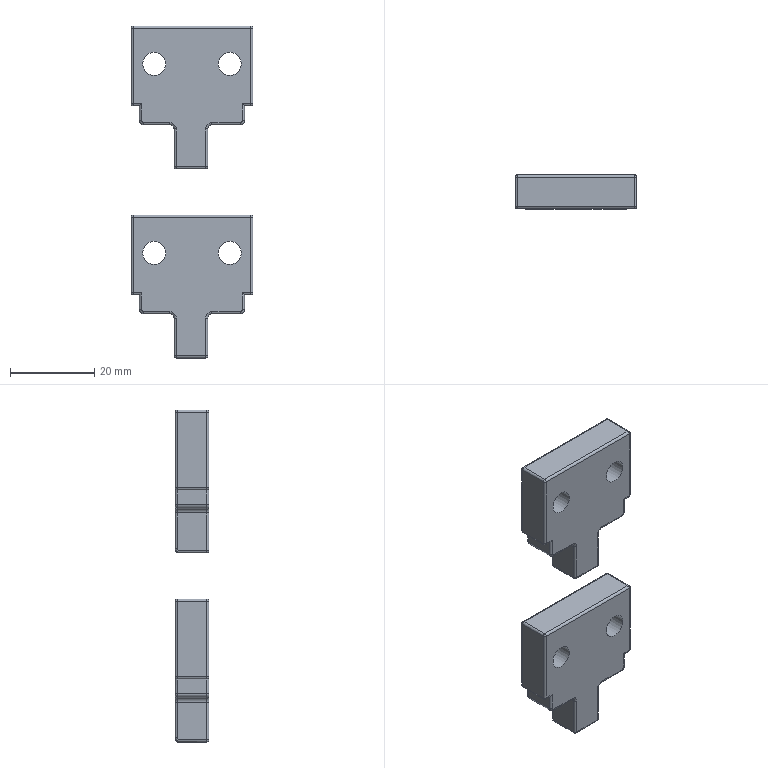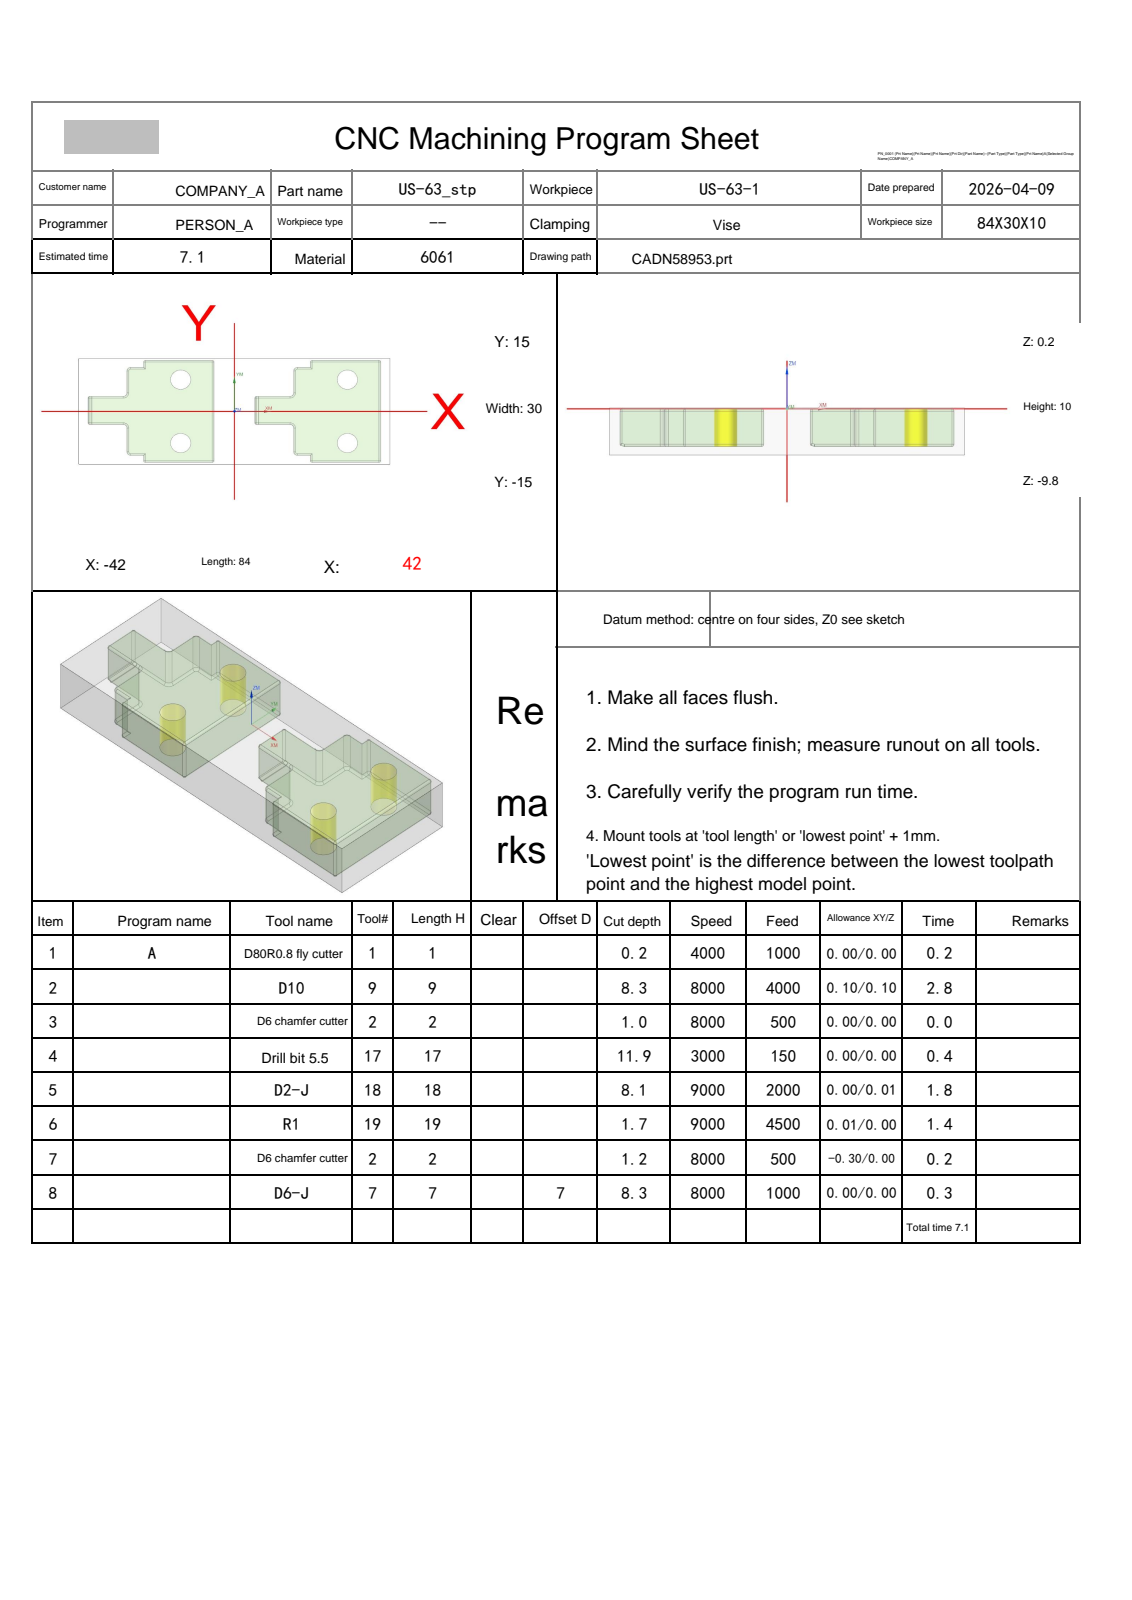NC program | NX | posted by the shop | part box 29 x 8 x 79 mm
Lines 2455 to 3429 of 24039:
N5 T18 M06
(D2-J  D=2. R=0. H=18 ce=0.00 di=0.01)
G00 G90 G54 X-24.921 Y-15.377 M03 S9000
G43 H18 Z20.
M08
Z.279
G01 X-24.92 Y-15.375 Z.232 F1600.
X-24.915 Y-15.367 Z.184
X-24.909 Y-15.355 Z.138
X-24.901 Y-15.339 Z.092
X-24.893 Y-15.319 Z.049
X-24.884 Y-15.297 Z.007
X-24.876 Y-15.272 Z-.031
X-24.869 Y-15.246 Z-.067
X-24.865 Y-15.219 Z-.1
X-24.863 Y-15.191 Z-.128
X-24.864 Y-15.163 Z-.152
X-24.869 Y-15.136 Z-.172
X-24.879 Y-15.11 Z-.187
X-24.894 Y-15.086 Z-.196
X-24.915 Y-15.063 Z-.199
G02 X-25.403 Y-14. I.915 J1.063 F2000.
G01 Y-13.403
X-28.
G02 X-28.256 Y-13.385 I0.0 J1.903
G01 X-28.273 Y-13.394 Z-.197
X-28.257 Y-13.426 Z-.193
X-28.213 Y-13.478 Z-.186
X-28.144 Y-13.548 Z-.178
X-28.052 Y-13.633 Z-.17
X-27.869 Y-13.785 Z-.159
X-27.735 Y-13.89 Z-.154
X-27.516 Y-14.051 Z-.151
X-27.144 Y-14.294 Z-.161
X-26.746 Y-14.522 Z-.187
X-26.337 Y-14.726 Z-.223
X-25.93 Y-14.897 Z-.267
X-25.676 Y-14.985 Z-.297
X-25.515 Y-15.035 Z-.317
X-25.289 Y-15.096 Z-.347
X-25.168 Y-15.123 Z-.363
X-25.073 Y-15.139 Z-.377
X-25.007 Y-15.145 Z-.388
X-24.974 Y-15.14 Z-.395
X-24.979 Y-15.124 Z-.398
G02 X-25.49 Y-14. I.979 J1.124
G01 Y-13.49
X-28.
G02 X-28.286 Y-13.47 I0.0 J1.99
G01 X-28.302 Y-13.478
X-28.287 Y-13.511
X-28.242 Y-13.565 Z-.399
X-28.172 Y-13.637 Z-.401
X-28.078 Y-13.724 Z-.403
X-27.893 Y-13.878 Z-.409
X-27.758 Y-13.984 Z-.414
X-27.535 Y-14.145 Z-.423
X-27.157 Y-14.385 Z-.444
X-26.753 Y-14.605 Z-.469
X-26.336 Y-14.798 Z-.498
X-25.923 Y-14.957 Z-.526
X-25.664 Y-15.038 Z-.544
X-25.501 Y-15.083 Z-.555
X-25.271 Y-15.137 Z-.571
X-25.149 Y-15.16 Z-.58
X-25.053 Y-15.173 Z-.587
X-24.985 Y-15.177 Z-.592
X-24.952 Y-15.171 Z-.595
X-24.957 Y-15.155 Z-.596
G02 X-25.5 Y-14. I.957 J1.155
G01 Y-13.5
X-28.
G02 X-28.284 Y-13.48 I0.0 J2.
G01 X-28.3 Y-13.486 Z-.597
X-28.29 Y-13.513 Z-.599
X-28.257 Y-13.557 Z-.602
X-28.201 Y-13.617 Z-.607
X-28.126 Y-13.689 Z-.612
X-27.924 Y-13.862 Z-.626
X-27.782 Y-13.975 Z-.635
X-27.534 Y-14.156 Z-.65
X-27.156 Y-14.394 Z-.672
X-26.752 Y-14.613 Z-.696
X-26.336 Y-14.805 Z-.719
X-25.922 Y-14.962 Z-.741
X-25.664 Y-15.042 Z-.755
X-25.501 Y-15.086 Z-.763
X-25.271 Y-15.139 Z-.776
X-25.149 Y-15.161 Z-.782
X-25.052 Y-15.174 Z-.787
X-24.985 Y-15.177 Z-.792
X-24.952 Y-15.171 Z-.794
X-24.957 Y-15.155 Z-.795
G02 X-25.5 Y-14. I.957 J1.155
G01 Y-13.5
X-28.
G02 X-28.285 Y-13.48 I0.0 J2.
G01 X-28.301 Y-13.486 Z-.796
X-28.291 Y-13.513 Z-.798
X-28.257 Y-13.557 Z-.801
X-28.201 Y-13.617 Z-.806
X-28.126 Y-13.689 Z-.811
X-27.925 Y-13.862 Z-.824
X-27.782 Y-13.975 Z-.834
X-27.534 Y-14.156 Z-.849
X-27.156 Y-14.394 Z-.871
X-26.752 Y-14.613 Z-.894
X-26.336 Y-14.805 Z-.918
X-25.922 Y-14.962 Z-.94
X-25.664 Y-15.042 Z-.954
X-25.501 Y-15.086 Z-.962
X-25.271 Y-15.139 Z-.974
X-25.149 Y-15.161 Z-.981
X-25.052 Y-15.174 Z-.986
X-24.985 Y-15.178 Z-.99
X-24.952 Y-15.171 Z-.993
X-24.957 Y-15.155 Z-.994
G02 X-25.5 Y-14. I.957 J1.155
G01 Y-13.5
X-28.
G02 X-28.285 Y-13.48 I0.0 J2.
G01 X-28.301 Y-13.486
X-28.291 Y-13.513 Z-.997
X-28.257 Y-13.557 Z-1.
X-28.201 Y-13.617 Z-1.004
X-28.126 Y-13.689 Z-1.01
X-27.925 Y-13.862 Z-1.023
X-27.782 Y-13.975 Z-1.032
X-27.534 Y-14.156 Z-1.048
X-27.156 Y-14.394 Z-1.07
X-26.752 Y-14.613 Z-1.093
X-26.336 Y-14.805 Z-1.116
X-25.922 Y-14.962 Z-1.139
X-25.664 Y-15.042 Z-1.152
X-25.501 Y-15.086 Z-1.161
X-25.271 Y-15.139 Z-1.173
X-25.149 Y-15.161 Z-1.18
X-25.052 Y-15.174 Z-1.185
X-24.985 Y-15.178 Z-1.189
X-24.952 Y-15.171 Z-1.192
X-24.957 Y-15.155 Z-1.193
G02 X-25.5 Y-14. I.957 J1.155
G01 Y-13.5
X-28.
G02 X-28.285 Y-13.48 I0.0 J2.
G01 X-28.301 Y-13.486
X-28.291 Y-13.513 Z-1.195
X-28.257 Y-13.557 Z-1.199
X-28.202 Y-13.617 Z-1.203
X-28.127 Y-13.689 Z-1.209
X-27.925 Y-13.862 Z-1.222
X-27.783 Y-13.975 Z-1.231
X-27.534 Y-14.156 Z-1.246
X-27.156 Y-14.394 Z-1.269
X-26.752 Y-14.613 Z-1.292
X-26.336 Y-14.805 Z-1.315
X-25.922 Y-14.962 Z-1.337
X-25.664 Y-15.042 Z-1.351
X-25.5 Y-15.086 Z-1.36
X-25.271 Y-15.139 Z-1.372
X-25.149 Y-15.161 Z-1.378
X-25.052 Y-15.174 Z-1.384
X-24.985 Y-15.178 Z-1.388
X-24.952 Y-15.171 Z-1.39
X-24.957 Y-15.155 Z-1.391
G02 X-25.5 Y-14. I.957 J1.155
G01 Y-13.5
X-28.
G02 X-28.285 Y-13.48 I0.0 J2.
G01 X-28.301 Y-13.486 Z-1.392
X-28.291 Y-13.513 Z-1.394
X-28.257 Y-13.557 Z-1.397
X-28.202 Y-13.617 Z-1.402
X-28.127 Y-13.689 Z-1.407
X-27.925 Y-13.862 Z-1.421
X-27.783 Y-13.975 Z-1.43
X-27.534 Y-14.156 Z-1.445
X-27.156 Y-14.394 Z-1.467
X-26.752 Y-14.613 Z-1.491
X-26.336 Y-14.805 Z-1.514
X-25.922 Y-14.962 Z-1.536
X-25.663 Y-15.042 Z-1.55
X-25.5 Y-15.086 Z-1.558
X-25.27 Y-15.139 Z-1.571
X-25.149 Y-15.161 Z-1.577
X-25.052 Y-15.174 Z-1.582
X-24.985 Y-15.178 Z-1.587
X-24.952 Y-15.171 Z-1.589
X-24.957 Y-15.155 Z-1.59
G02 X-25.5 Y-14. I.957 J1.155
G01 Y-13.5
X-28.
G02 X-28.286 Y-13.48 I0.0 J2.
G01 X-28.302 Y-13.486 Z-1.591
X-28.292 Y-13.513 Z-1.593
X-28.258 Y-13.557 Z-1.596
X-28.202 Y-13.617 Z-1.601
X-28.127 Y-13.689 Z-1.606
X-27.925 Y-13.862 Z-1.619
X-27.783 Y-13.975 Z-1.629
X-27.534 Y-14.156 Z-1.644
X-27.156 Y-14.394 Z-1.666
X-26.752 Y-14.613 Z-1.689
X-26.336 Y-14.805 Z-1.713
X-25.922 Y-14.962 Z-1.735
X-25.663 Y-15.042 Z-1.749
X-25.5 Y-15.086 Z-1.757
X-25.27 Y-15.139 Z-1.769
X-25.149 Y-15.161 Z-1.776
X-25.052 Y-15.174 Z-1.781
X-24.985 Y-15.178 Z-1.785
X-24.952 Y-15.172 Z-1.788
X-24.957 Y-15.155 Z-1.789
G02 X-25.5 Y-14. I.957 J1.155
G01 Y-13.5
X-28.
G02 X-28.286 Y-13.479 I0.0 J2.
G01 X-28.302 Y-13.486
X-28.292 Y-13.513 Z-1.792
X-28.258 Y-13.557 Z-1.795
X-28.202 Y-13.617 Z-1.799
X-28.127 Y-13.689 Z-1.805
X-27.925 Y-13.862 Z-1.818
X-27.783 Y-13.974 Z-1.827
X-27.534 Y-14.156 Z-1.843
X-27.157 Y-14.394 Z-1.865
X-26.752 Y-14.613 Z-1.888
X-26.336 Y-14.805 Z-1.911
X-25.922 Y-14.962 Z-1.934
X-25.663 Y-15.042 Z-1.947
X-25.5 Y-15.086 Z-1.956
X-25.27 Y-15.139 Z-1.968
X-25.148 Y-15.162 Z-1.975
X-25.052 Y-15.174 Z-1.98
X-24.985 Y-15.178 Z-1.984
X-24.951 Y-15.172 Z-1.987
X-24.957 Y-15.155 Z-1.988
G02 X-25.5 Y-14. I.957 J1.155
G01 Y-13.5
X-28.
G02 X-28.286 Y-13.479 I0.0 J2.
G01 X-28.302 Y-13.486
X-28.292 Y-13.513 Z-1.99
X-28.258 Y-13.557 Z-1.994
X-28.202 Y-13.617 Z-1.998
X-28.127 Y-13.689 Z-2.004
X-27.926 Y-13.862 Z-2.017
X-27.783 Y-13.974 Z-2.026
X-27.535 Y-14.156 Z-2.041
X-27.157 Y-14.394 Z-2.064
X-26.752 Y-14.613 Z-2.087
X-26.336 Y-14.805 Z-2.11
X-25.922 Y-14.962 Z-2.132
X-25.663 Y-15.042 Z-2.146
X-25.5 Y-15.086 Z-2.155
X-25.27 Y-15.139 Z-2.167
X-25.148 Y-15.162 Z-2.173
X-25.052 Y-15.175 Z-2.179
X-24.985 Y-15.178 Z-2.183
X-24.951 Y-15.172 Z-2.185
X-24.956 Y-15.156 Z-2.186
G02 X-25.5 Y-14. I.956 J1.156
G01 Y-13.5
X-28.
G02 X-28.286 Y-13.479 I0.0 J2.
G01 X-28.302 Y-13.486 Z-2.187
X-28.292 Y-13.513 Z-2.189
X-28.258 Y-13.557 Z-2.192
X-28.203 Y-13.617 Z-2.197
X-28.128 Y-13.689 Z-2.202
X-27.926 Y-13.862 Z-2.216
X-27.783 Y-13.974 Z-2.225
X-27.535 Y-14.156 Z-2.24
X-27.157 Y-14.394 Z-2.262
X-26.752 Y-14.613 Z-2.286
X-26.336 Y-14.805 Z-2.309
X-25.922 Y-14.962 Z-2.331
X-25.663 Y-15.042 Z-2.345
X-25.5 Y-15.086 Z-2.353
X-25.27 Y-15.139 Z-2.366
X-25.148 Y-15.162 Z-2.372
X-25.052 Y-15.175 Z-2.377
X-24.984 Y-15.178 Z-2.382
X-24.951 Y-15.172 Z-2.384
X-24.956 Y-15.156 Z-2.385
G02 X-25.5 Y-14. I.956 J1.156
G01 Y-13.5
X-28.
G02 X-28.287 Y-13.479 I0.0 J2.
G01 X-28.302 Y-13.486 Z-2.386
X-28.292 Y-13.513 Z-2.388
X-28.259 Y-13.557 Z-2.391
X-28.203 Y-13.617 Z-2.396
X-28.128 Y-13.689 Z-2.401
X-27.926 Y-13.862 Z-2.414
X-27.784 Y-13.974 Z-2.424
X-27.535 Y-14.156 Z-2.439
X-27.157 Y-14.394 Z-2.461
X-26.752 Y-14.613 Z-2.484
X-26.336 Y-14.805 Z-2.508
X-25.922 Y-14.962 Z-2.53
X-25.663 Y-15.042 Z-2.544
X-25.5 Y-15.086 Z-2.552
X-25.27 Y-15.14 Z-2.564
X-25.148 Y-15.162 Z-2.571
X-25.052 Y-15.175 Z-2.576
X-24.984 Y-15.178 Z-2.58
X-24.951 Y-15.172 Z-2.583
X-24.956 Y-15.156 Z-2.584
G02 X-25.5 Y-14. I.956 J1.156
G01 Y-13.5
X-28.
G02 X-28.287 Y-13.479 I0.0 J2.
G01 X-28.303 Y-13.486
X-28.293 Y-13.513 Z-2.587
X-28.259 Y-13.557 Z-2.59
X-28.203 Y-13.617 Z-2.594
X-28.128 Y-13.689 Z-2.6
X-27.926 Y-13.862 Z-2.613
X-27.784 Y-13.974 Z-2.622
X-27.535 Y-14.156 Z-2.638
X-27.157 Y-14.394 Z-2.66
X-26.753 Y-14.613 Z-2.683
X-26.336 Y-14.805 Z-2.706
X-25.922 Y-14.962 Z-2.729
X-25.663 Y-15.042 Z-2.742
X-25.5 Y-15.086 Z-2.751
X-25.27 Y-15.14 Z-2.763
X-25.148 Y-15.162 Z-2.77
X-25.051 Y-15.175 Z-2.775
X-24.984 Y-15.178 Z-2.779
X-24.951 Y-15.172 Z-2.782
X-24.956 Y-15.156 Z-2.783
G02 X-25.5 Y-14. I.956 J1.156
G01 Y-13.5
X-28.
G02 X-28.287 Y-13.479 I0.0 J2.
G01 X-28.303 Y-13.486
X-28.293 Y-13.513 Z-2.785
X-28.259 Y-13.557 Z-2.789
X-28.203 Y-13.617 Z-2.793
X-28.128 Y-13.689 Z-2.799
X-27.926 Y-13.862 Z-2.812
X-27.784 Y-13.974 Z-2.821
X-27.535 Y-14.156 Z-2.836
X-27.157 Y-14.394 Z-2.859
X-26.753 Y-14.613 Z-2.882
X-26.336 Y-14.805 Z-2.905
X-25.922 Y-14.962 Z-2.927
X-25.663 Y-15.042 Z-2.941
X-25.5 Y-15.086 Z-2.95
X-25.27 Y-15.14 Z-2.962
X-25.148 Y-15.162 Z-2.968
X-25.051 Y-15.175 Z-2.974
X-24.984 Y-15.178 Z-2.978
X-24.951 Y-15.172 Z-2.98
X-24.956 Y-15.156 Z-2.981
G02 X-25.5 Y-14. I.956 J1.156
G01 Y-13.5
X-28.
G02 X-28.287 Y-13.479 I0.0 J2.
G01 X-28.303 Y-13.486 Z-2.982
X-28.293 Y-13.513 Z-2.984
X-28.259 Y-13.557 Z-2.987
X-28.204 Y-13.617 Z-2.992
X-28.128 Y-13.689 Z-2.997
X-27.927 Y-13.862 Z-3.011
X-27.784 Y-13.974 Z-3.02
X-27.535 Y-14.156 Z-3.035
X-27.157 Y-14.394 Z-3.057
X-26.753 Y-14.613 Z-3.081
X-26.336 Y-14.805 Z-3.104
X-25.922 Y-14.962 Z-3.126
X-25.663 Y-15.042 Z-3.14
X-25.5 Y-15.086 Z-3.148
X-25.27 Y-15.14 Z-3.161
X-25.148 Y-15.162 Z-3.167
X-25.051 Y-15.175 Z-3.172
X-24.984 Y-15.178 Z-3.177
X-24.951 Y-15.172 Z-3.179
X-24.956 Y-15.156 Z-3.18
G02 X-25.5 Y-14. I.956 J1.156
G01 Y-13.5
X-28.
G02 X-28.287 Y-13.479 I0.0 J2.
G01 X-28.303 Y-13.486 Z-3.181
X-28.293 Y-13.513 Z-3.183
X-28.259 Y-13.557 Z-3.186
X-28.204 Y-13.617 Z-3.191
X-28.129 Y-13.689 Z-3.196
X-27.927 Y-13.862 Z-3.209
X-27.784 Y-13.974 Z-3.219
X-27.535 Y-14.156 Z-3.234
X-27.157 Y-14.394 Z-3.256
X-26.753 Y-14.613 Z-3.279
X-26.336 Y-14.805 Z-3.303
X-25.922 Y-14.962 Z-3.325
X-25.663 Y-15.042 Z-3.339
X-25.5 Y-15.086 Z-3.347
X-25.27 Y-15.14 Z-3.359
X-25.148 Y-15.162 Z-3.366
X-25.051 Y-15.175 Z-3.371
X-24.984 Y-15.178 Z-3.375
X-24.951 Y-15.172 Z-3.378
X-24.956 Y-15.156 Z-3.379
G02 X-25.5 Y-14. I.956 J1.156
G01 Y-13.5
X-28.
G02 X-28.288 Y-13.479 I0.0 J2.
G01 X-28.304 Y-13.486
X-28.294 Y-13.512 Z-3.382
X-28.26 Y-13.557 Z-3.385
X-28.204 Y-13.616 Z-3.389
X-28.129 Y-13.689 Z-3.395
X-27.927 Y-13.862 Z-3.408
X-27.784 Y-13.974 Z-3.417
X-27.536 Y-14.156 Z-3.433
X-27.157 Y-14.394 Z-3.455
X-26.753 Y-14.613 Z-3.478
X-26.336 Y-14.805 Z-3.501
X-25.922 Y-14.962 Z-3.524
X-25.663 Y-15.042 Z-3.537
X-25.5 Y-15.087 Z-3.546
X-25.27 Y-15.14 Z-3.558
X-25.148 Y-15.162 Z-3.565
X-25.051 Y-15.175 Z-3.57
X-24.984 Y-15.179 Z-3.574
X-24.951 Y-15.172 Z-3.577
X-24.956 Y-15.156 Z-3.578
G02 X-25.5 Y-14. I.956 J1.156
G01 Y-13.5
X-28.
G02 X-28.288 Y-13.479 I0.0 J2.
G01 X-28.304 Y-13.486
X-28.294 Y-13.512 Z-3.58
X-28.26 Y-13.557 Z-3.584
X-28.204 Y-13.616 Z-3.588
X-28.129 Y-13.689 Z-3.594
X-27.927 Y-13.862 Z-3.607
X-27.785 Y-13.974 Z-3.616
X-27.536 Y-14.156 Z-3.631
X-27.158 Y-14.394 Z-3.654
X-26.753 Y-14.613 Z-3.677
X-26.336 Y-14.805 Z-3.7
X-25.922 Y-14.962 Z-3.722
X-25.663 Y-15.042 Z-3.736
X-25.5 Y-15.087 Z-3.745
X-25.27 Y-15.14 Z-3.757
X-25.148 Y-15.162 Z-3.763
X-25.051 Y-15.175 Z-3.769
X-24.984 Y-15.179 Z-3.773
X-24.951 Y-15.172 Z-3.775
X-24.956 Y-15.156 Z-3.776
G02 X-25.5 Y-14. I.956 J1.156
G01 Y-13.5
X-28.
G02 X-28.288 Y-13.479 I0.0 J2.
G01 X-28.304 Y-13.486 Z-3.777
X-28.294 Y-13.512 Z-3.779
X-28.26 Y-13.557 Z-3.782
X-28.204 Y-13.616 Z-3.787
X-28.129 Y-13.689 Z-3.792
X-27.927 Y-13.862 Z-3.806
X-27.785 Y-13.974 Z-3.815
X-27.536 Y-14.156 Z-3.83
X-27.158 Y-14.394 Z-3.852
X-26.753 Y-14.613 Z-3.876
X-26.336 Y-14.805 Z-3.899
X-25.922 Y-14.963 Z-3.921
X-25.663 Y-15.042 Z-3.935
X-25.5 Y-15.087 Z-3.943
X-25.27 Y-15.14 Z-3.956
X-25.148 Y-15.162 Z-3.962
X-25.051 Y-15.175 Z-3.967
X-24.984 Y-15.179 Z-3.972
X-24.95 Y-15.172 Z-3.974
X-24.956 Y-15.156 Z-3.975
G02 X-25.5 Y-14. I.956 J1.156
G01 Y-13.5
X-28.
G02 X-28.288 Y-13.479 I0.0 J2.
G01 X-28.304 Y-13.486 Z-3.976
X-28.294 Y-13.512 Z-3.978
X-28.26 Y-13.557 Z-3.981
X-28.204 Y-13.617 Z-3.986
X-28.129 Y-13.689 Z-3.991
X-27.927 Y-13.862 Z-4.004
X-27.784 Y-13.975 Z-4.014
X-27.534 Y-14.156 Z-4.029
X-27.156 Y-14.396 Z-4.051
X-26.75 Y-14.615 Z-4.074
X-26.333 Y-14.807 Z-4.098
X-25.918 Y-14.965 Z-4.12
X-25.659 Y-15.045 Z-4.134
X-25.496 Y-15.09 Z-4.142
X-25.265 Y-15.143 Z-4.154
X-25.143 Y-15.165 Z-4.161
X-25.046 Y-15.179 Z-4.166
X-24.979 Y-15.182 Z-4.17
X-24.946 Y-15.176 Z-4.173
X-24.951 Y-15.16 Z-4.174
G02 X-25.5 Y-14. I.951 J1.16
G01 Y-13.5
X-28.
G02 X-28.298 Y-13.478 I0.0 J2.
G01 X-28.314 Y-13.484
X-28.304 Y-13.511 Z-4.177
X-28.269 Y-13.555 Z-4.18
X-28.214 Y-13.615 Z-4.184
X-28.138 Y-13.687 Z-4.19
X-27.935 Y-13.861 Z-4.203
X-27.792 Y-13.973 Z-4.212
X-27.542 Y-14.155 Z-4.228
X-27.162 Y-14.394 Z-4.25
X-26.756 Y-14.614 Z-4.273
X-26.337 Y-14.806 Z-4.296
X-25.921 Y-14.964 Z-4.319
X-25.661 Y-15.045 Z-4.332
X-25.497 Y-15.089 Z-4.341
X-25.266 Y-15.143 Z-4.353
X-25.144 Y-15.165 Z-4.36
X-25.047 Y-15.178 Z-4.365
X-24.979 Y-15.182 Z-4.369
X-24.946 Y-15.176 Z-4.372
X-24.951 Y-15.16 Z-4.373
G02 X-25.5 Y-14. I.951 J1.16
G01 Y-13.5
X-28.
G02 X-28.298 Y-13.478 I0.0 J2.
G01 X-28.314 Y-13.484
X-28.304 Y-13.511 Z-4.375
X-28.269 Y-13.555 Z-4.379
X-28.214 Y-13.615 Z-4.383
X-28.138 Y-13.687 Z-4.389
X-27.935 Y-13.861 Z-4.402
X-27.792 Y-13.973 Z-4.411
X-27.542 Y-14.155 Z-4.426
X-27.162 Y-14.394 Z-4.449
X-26.756 Y-14.614 Z-4.472
X-26.337 Y-14.806 Z-4.495
X-25.921 Y-14.964 Z-4.517
X-25.661 Y-15.045 Z-4.531
X-25.497 Y-15.089 Z-4.54
X-25.266 Y-15.143 Z-4.552
X-25.144 Y-15.165 Z-4.558
X-25.047 Y-15.178 Z-4.564
X-24.979 Y-15.182 Z-4.568
X-24.946 Y-15.176 Z-4.57
X-24.951 Y-15.16 Z-4.571
G02 X-25.5 Y-14. I.951 J1.16
G01 Y-13.5
X-28.
G02 X-28.298 Y-13.478 I0.0 J2.
G01 X-28.314 Y-13.484 Z-4.572
X-28.304 Y-13.511 Z-4.574
X-28.269 Y-13.555 Z-4.577
X-28.214 Y-13.615 Z-4.582
X-28.138 Y-13.687 Z-4.587
X-27.935 Y-13.861 Z-4.601
X-27.792 Y-13.973 Z-4.61
X-27.542 Y-14.155 Z-4.625
X-27.162 Y-14.394 Z-4.647
X-26.756 Y-14.614 Z-4.671
X-26.337 Y-14.806 Z-4.694
X-25.921 Y-14.964 Z-4.716
X-25.661 Y-15.045 Z-4.73
X-25.497 Y-15.089 Z-4.738
X-25.266 Y-15.143 Z-4.751
X-25.144 Y-15.165 Z-4.757
X-25.047 Y-15.178 Z-4.762
X-24.979 Y-15.182 Z-4.767
X-24.946 Y-15.176 Z-4.769
X-24.951 Y-15.16 Z-4.77
G02 X-25.5 Y-14. I.951 J1.16
G01 Y-13.5
X-28.
G02 X-28.298 Y-13.478 I0.0 J2.
G01 X-28.314 Y-13.484 Z-4.771
X-28.304 Y-13.511 Z-4.773
X-28.269 Y-13.555 Z-4.776
X-28.214 Y-13.615 Z-4.781
X-28.138 Y-13.687 Z-4.786
X-27.935 Y-13.861 Z-4.799
X-27.792 Y-13.973 Z-4.809
X-27.542 Y-14.155 Z-4.824
X-27.162 Y-14.394 Z-4.846
X-26.756 Y-14.614 Z-4.869
X-26.337 Y-14.806 Z-4.893
X-25.921 Y-14.964 Z-4.915
X-25.661 Y-15.045 Z-4.929
X-25.497 Y-15.089 Z-4.937
X-25.266 Y-15.143 Z-4.949
X-25.144 Y-15.165 Z-4.956
X-25.047 Y-15.178 Z-4.961
X-24.979 Y-15.182 Z-4.965
X-24.946 Y-15.176 Z-4.968
X-24.951 Y-15.16 Z-4.969
G02 X-25.5 Y-14. I.951 J1.16
G01 Y-13.5
X-28.
G02 X-28.298 Y-13.478 I0.0 J2.
G01 X-28.314 Y-13.484
X-28.304 Y-13.511 Z-4.972
X-28.269 Y-13.555 Z-4.975
X-28.214 Y-13.615 Z-4.979
X-28.138 Y-13.687 Z-4.985
X-27.935 Y-13.861 Z-4.998
X-27.792 Y-13.973 Z-5.007
X-27.542 Y-14.155 Z-5.023
X-27.162 Y-14.394 Z-5.045
X-26.756 Y-14.614 Z-5.068
X-26.337 Y-14.806 Z-5.091
X-25.921 Y-14.964 Z-5.114
X-25.661 Y-15.045 Z-5.127
X-25.497 Y-15.089 Z-5.136
X-25.266 Y-15.143 Z-5.148
X-25.144 Y-15.165 Z-5.155
X-25.047 Y-15.178 Z-5.16
X-24.979 Y-15.182 Z-5.164
X-24.946 Y-15.176 Z-5.167
X-24.951 Y-15.16 Z-5.168
G02 X-25.5 Y-14. I.951 J1.16
G01 Y-13.5
X-28.
G02 X-28.298 Y-13.478 I0.0 J2.
G01 X-28.314 Y-13.484
X-28.304 Y-13.511 Z-5.17
X-28.269 Y-13.555 Z-5.174
X-28.214 Y-13.615 Z-5.178
X-28.138 Y-13.687 Z-5.184
X-27.935 Y-13.861 Z-5.197
X-27.792 Y-13.973 Z-5.206
X-27.542 Y-14.155 Z-5.221
X-27.162 Y-14.394 Z-5.244
X-26.756 Y-14.614 Z-5.267
X-26.337 Y-14.806 Z-5.29
X-25.921 Y-14.964 Z-5.312
X-25.661 Y-15.045 Z-5.326
X-25.497 Y-15.089 Z-5.335
X-25.266 Y-15.143 Z-5.347
X-25.144 Y-15.165 Z-5.353
X-25.047 Y-15.178 Z-5.359
X-24.979 Y-15.182 Z-5.363
X-24.946 Y-15.176 Z-5.365
X-24.951 Y-15.16 Z-5.366
G02 X-25.5 Y-14. I.951 J1.16
G01 Y-13.5
X-28.
G02 X-28.298 Y-13.478 I0.0 J2.
G01 X-28.314 Y-13.484 Z-5.367
X-28.304 Y-13.511 Z-5.369
X-28.269 Y-13.555 Z-5.372
X-28.214 Y-13.615 Z-5.377
X-28.138 Y-13.687 Z-5.382
X-27.935 Y-13.861 Z-5.396
X-27.792 Y-13.973 Z-5.405
X-27.542 Y-14.155 Z-5.42
X-27.162 Y-14.394 Z-5.442
X-26.756 Y-14.614 Z-5.466
X-26.337 Y-14.806 Z-5.489
X-25.921 Y-14.964 Z-5.511
X-25.661 Y-15.045 Z-5.525
X-25.497 Y-15.089 Z-5.533
X-25.266 Y-15.143 Z-5.546
X-25.144 Y-15.165 Z-5.552
X-25.047 Y-15.178 Z-5.557
X-24.979 Y-15.182 Z-5.562
X-24.946 Y-15.176 Z-5.564
X-24.951 Y-15.16 Z-5.565
G02 X-25.5 Y-14. I.951 J1.16
G01 Y-13.5
X-28.
G02 X-28.298 Y-13.478 I0.0 J2.
G01 X-28.314 Y-13.484 Z-5.566
X-28.304 Y-13.511 Z-5.568
X-28.269 Y-13.555 Z-5.571
X-28.214 Y-13.615 Z-5.576
X-28.138 Y-13.687 Z-5.581
X-27.935 Y-13.861 Z-5.594
X-27.792 Y-13.973 Z-5.604
X-27.542 Y-14.155 Z-5.619
X-27.162 Y-14.394 Z-5.641
X-26.756 Y-14.614 Z-5.664
X-26.337 Y-14.806 Z-5.688
X-25.921 Y-14.964 Z-5.71
X-25.661 Y-15.045 Z-5.724
X-25.497 Y-15.089 Z-5.732
X-25.266 Y-15.143 Z-5.744
X-25.144 Y-15.165 Z-5.751
X-25.047 Y-15.178 Z-5.756
X-24.979 Y-15.182 Z-5.76
X-24.946 Y-15.176 Z-5.763
X-24.951 Y-15.16 Z-5.764
G02 X-25.5 Y-14. I.951 J1.16
G01 Y-13.5
X-28.
G02 X-28.298 Y-13.478 I0.0 J2.
G01 X-28.314 Y-13.484
X-28.304 Y-13.511 Z-5.767
X-28.269 Y-13.555 Z-5.77
X-28.214 Y-13.615 Z-5.774
X-28.138 Y-13.687 Z-5.78
X-27.935 Y-13.861 Z-5.793
X-27.792 Y-13.973 Z-5.802
X-27.542 Y-14.155 Z-5.818
X-27.162 Y-14.394 Z-5.84
X-26.756 Y-14.614 Z-5.863
X-26.337 Y-14.806 Z-5.886
X-25.921 Y-14.964 Z-5.909
X-25.661 Y-15.045 Z-5.922
X-25.497 Y-15.089 Z-5.931
X-25.266 Y-15.143 Z-5.943
X-25.144 Y-15.165 Z-5.95
X-25.047 Y-15.178 Z-5.955
X-24.979 Y-15.182 Z-5.959
X-24.946 Y-15.176 Z-5.962
X-24.951 Y-15.16 Z-5.963
G02 X-25.5 Y-14. I.951 J1.16
G01 Y-13.5
X-28.
G02 X-28.298 Y-13.478 I0.0 J2.
G01 X-28.314 Y-13.484
X-28.304 Y-13.511 Z-5.965
X-28.269 Y-13.555 Z-5.969
X-28.214 Y-13.615 Z-5.973
X-28.138 Y-13.687 Z-5.979
X-27.935 Y-13.861 Z-5.992
X-27.792 Y-13.973 Z-6.001
X-27.542 Y-14.155 Z-6.016
X-27.162 Y-14.394 Z-6.039
X-26.756 Y-14.614 Z-6.062
X-26.337 Y-14.806 Z-6.085
X-25.921 Y-14.964 Z-6.107
X-25.661 Y-15.045 Z-6.121
X-25.497 Y-15.089 Z-6.13
X-25.266 Y-15.143 Z-6.142
X-25.144 Y-15.165 Z-6.148
X-25.047 Y-15.178 Z-6.154
X-24.979 Y-15.182 Z-6.158
X-24.946 Y-15.176 Z-6.16
X-24.951 Y-15.16 Z-6.161
G02 X-25.5 Y-14. I.951 J1.16
G01 Y-13.5
X-28.
G02 X-28.298 Y-13.478 I0.0 J2.
G01 X-28.314 Y-13.484 Z-6.162
X-28.304 Y-13.511 Z-6.164
X-28.269 Y-13.555 Z-6.167
X-28.214 Y-13.615 Z-6.172
X-28.138 Y-13.687 Z-6.177
X-27.935 Y-13.861 Z-6.191
X-27.792 Y-13.973 Z-6.2
X-27.542 Y-14.155 Z-6.215
X-27.162 Y-14.394 Z-6.237
X-26.756 Y-14.614 Z-6.261
X-26.337 Y-14.806 Z-6.284
X-25.921 Y-14.964 Z-6.306
X-25.661 Y-15.045 Z-6.32
X-25.497 Y-15.089 Z-6.328
X-25.266 Y-15.143 Z-6.341
X-25.144 Y-15.165 Z-6.347
X-25.047 Y-15.178 Z-6.352
X-24.979 Y-15.182 Z-6.357
X-24.946 Y-15.176 Z-6.359
X-24.951 Y-15.16 Z-6.36
G02 X-25.5 Y-14. I.951 J1.16
G01 Y-13.5
X-28.
G02 X-28.298 Y-13.478 I0.0 J2.
G01 X-28.314 Y-13.484 Z-6.361
X-28.304 Y-13.511 Z-6.363
X-28.269 Y-13.555 Z-6.366
X-28.214 Y-13.615 Z-6.371
X-28.138 Y-13.687 Z-6.376
X-27.935 Y-13.861 Z-6.389
X-27.792 Y-13.973 Z-6.399
X-27.542 Y-14.155 Z-6.414
X-27.162 Y-14.394 Z-6.436
X-26.756 Y-14.614 Z-6.459
X-26.337 Y-14.806 Z-6.483
X-25.921 Y-14.964 Z-6.505
X-25.661 Y-15.045 Z-6.519
X-25.497 Y-15.089 Z-6.527
X-25.266 Y-15.143 Z-6.539
X-25.144 Y-15.165 Z-6.546
X-25.047 Y-15.178 Z-6.551
X-24.979 Y-15.182 Z-6.555
X-24.946 Y-15.176 Z-6.558
X-24.951 Y-15.16 Z-6.559
G02 X-25.5 Y-14. I.951 J1.16
G01 Y-13.5
X-28.
G02 X-28.298 Y-13.478 I0.0 J2.
G01 X-28.314 Y-13.484
X-28.304 Y-13.511 Z-6.562
X-28.269 Y-13.555 Z-6.565
X-28.214 Y-13.615 Z-6.569
X-28.138 Y-13.687 Z-6.575
X-27.935 Y-13.861 Z-6.588
X-27.792 Y-13.973 Z-6.597
X-27.542 Y-14.155 Z-6.613
X-27.162 Y-14.394 Z-6.635
X-26.756 Y-14.614 Z-6.658
X-26.337 Y-14.806 Z-6.681
X-25.921 Y-14.964 Z-6.704
X-25.661 Y-15.045 Z-6.717
X-25.497 Y-15.089 Z-6.726
X-25.266 Y-15.143 Z-6.738
X-25.144 Y-15.165 Z-6.745
X-25.047 Y-15.178 Z-6.75
X-24.979 Y-15.182 Z-6.754
X-24.946 Y-15.176 Z-6.757
X-24.951 Y-15.16 Z-6.758
G02 X-25.5 Y-14. I.951 J1.16
G01 Y-13.5
X-28.
G02 X-28.298 Y-13.478 I0.0 J2.
G01 X-28.314 Y-13.484
X-28.304 Y-13.511 Z-6.76
X-28.269 Y-13.555 Z-6.764
X-28.214 Y-13.615 Z-6.768
X-28.138 Y-13.687 Z-6.774
X-27.935 Y-13.861 Z-6.787
X-27.792 Y-13.973 Z-6.796
X-27.542 Y-14.155 Z-6.811
X-27.162 Y-14.394 Z-6.834
X-26.756 Y-14.614 Z-6.857
X-26.337 Y-14.806 Z-6.88
X-25.921 Y-14.964 Z-6.902
X-25.661 Y-15.045 Z-6.916
X-25.497 Y-15.089 Z-6.925
X-25.266 Y-15.143 Z-6.937
X-25.144 Y-15.165 Z-6.943
X-25.047 Y-15.178 Z-6.949
X-24.979 Y-15.182 Z-6.953
X-24.946 Y-15.176 Z-6.955
X-24.951 Y-15.16 Z-6.956
G02 X-25.5 Y-14. I.951 J1.16
G01 Y-13.5
X-28.
G02 X-28.298 Y-13.478 I0.0 J2.
G01 X-28.314 Y-13.484 Z-6.957
X-28.304 Y-13.511 Z-6.959
X-28.269 Y-13.555 Z-6.962
X-28.214 Y-13.615 Z-6.967
X-28.138 Y-13.687 Z-6.972
X-27.935 Y-13.861 Z-6.986
X-27.792 Y-13.973 Z-6.995
X-27.542 Y-14.155 Z-7.01
X-27.162 Y-14.394 Z-7.032
X-26.756 Y-14.614 Z-7.056
X-26.337 Y-14.806 Z-7.079
X-25.921 Y-14.964 Z-7.101
X-25.661 Y-15.045 Z-7.115
X-25.497 Y-15.089 Z-7.123
X-25.266 Y-15.143 Z-7.136
X-25.144 Y-15.165 Z-7.142
X-25.047 Y-15.178 Z-7.147
X-24.979 Y-15.182 Z-7.152
X-24.946 Y-15.176 Z-7.154
X-24.951 Y-15.16 Z-7.155
G02 X-25.5 Y-14. I.951 J1.16
G01 Y-13.5
X-28.
G02 X-28.298 Y-13.478 I0.0 J2.
G01 X-28.314 Y-13.484 Z-7.156
X-28.304 Y-13.511 Z-7.158
X-28.269 Y-13.555 Z-7.161
X-28.214 Y-13.615 Z-7.166
X-28.138 Y-13.687 Z-7.171
X-27.935 Y-13.861 Z-7.184
X-27.792 Y-13.973 Z-7.194
X-27.542 Y-14.155 Z-7.209
X-27.162 Y-14.394 Z-7.231
X-26.756 Y-14.614 Z-7.254
X-26.337 Y-14.806 Z-7.278
X-25.921 Y-14.964 Z-7.3
X-25.661 Y-15.045 Z-7.314
X-25.497 Y-15.089 Z-7.322
X-25.266 Y-15.143 Z-7.334
X-25.144 Y-15.165 Z-7.341
X-25.047 Y-15.178 Z-7.346
X-24.979 Y-15.182 Z-7.35
X-24.946 Y-15.176 Z-7.353
X-24.951 Y-15.16 Z-7.354
G02 X-25.5 Y-14. I.951 J1.16
G01 Y-13.5
X-28.
G02 X-28.298 Y-13.478 I0.0 J2.
G01 X-28.314 Y-13.484
X-28.304 Y-13.511 Z-7.357
X-28.269 Y-13.555 Z-7.36
X-28.214 Y-13.615 Z-7.364
X-28.138 Y-13.687 Z-7.37
X-27.935 Y-13.861 Z-7.383
X-27.792 Y-13.973 Z-7.392
X-27.542 Y-14.155 Z-7.408
X-27.162 Y-14.394 Z-7.43
X-26.756 Y-14.614 Z-7.453
X-26.337 Y-14.806 Z-7.476
X-25.921 Y-14.965 Z-7.499
X-25.661 Y-15.045 Z-7.512
X-25.497 Y-15.089 Z-7.521
X-25.266 Y-15.143 Z-7.533
X-25.144 Y-15.165 Z-7.54
X-25.047 Y-15.179 Z-7.545
X-24.979 Y-15.182 Z-7.549
X-24.946 Y-15.176 Z-7.552
X-24.951 Y-15.16 Z-7.553
G02 X-25.5 Y-14. I.951 J1.16
G01 Y-13.5
X-28.
G02 X-28.298 Y-13.478 I0.0 J2.
G01 X-28.314 Y-13.484
X-28.304 Y-13.511 Z-7.555
X-28.27 Y-13.555 Z-7.559
X-28.214 Y-13.615 Z-7.563
X-28.138 Y-13.687 Z-7.569
X-27.935 Y-13.861 Z-7.582
X-27.792 Y-13.973 Z-7.591
X-27.542 Y-14.155 Z-7.606
X-27.162 Y-14.394 Z-7.629
X-26.756 Y-14.614 Z-7.652
X-26.337 Y-14.806 Z-7.675
X-25.921 Y-14.964 Z-7.697
X-25.661 Y-15.045 Z-7.711
X-25.497 Y-15.089 Z-7.72
X-25.266 Y-15.143 Z-7.732
X-25.144 Y-15.165 Z-7.738
X-25.047 Y-15.179 Z-7.744
X-24.979 Y-15.182 Z-7.748
X-24.946 Y-15.176 Z-7.75
X-24.951 Y-15.16 Z-7.751
G02 X-25.5 Y-14. I.951 J1.16
G01 Y-13.5
X-28.
G02 X-28.298 Y-13.478 I0.0 J2.
G01 X-28.314 Y-13.484 Z-7.752
X-28.304 Y-13.511 Z-7.754
X-28.27 Y-13.555 Z-7.757
X-28.214 Y-13.615 Z-7.762
X-28.138 Y-13.687 Z-7.767
X-27.935 Y-13.861 Z-7.781
X-27.792 Y-13.973 Z-7.79
X-27.542 Y-14.155 Z-7.805
X-27.162 Y-14.394 Z-7.827
X-26.756 Y-14.614 Z-7.851
X-26.337 Y-14.806 Z-7.874
X-25.921 Y-14.964 Z-7.896
X-25.661 Y-15.045 Z-7.91
X-25.497 Y-15.089 Z-7.918
X-25.266 Y-15.143 Z-7.931
X-25.144 Y-15.165 Z-7.937
X-25.047 Y-15.179 Z-7.942
X-24.979 Y-15.182 Z-7.947
X-24.946 Y-15.176 Z-7.949
X-24.951 Y-15.16 Z-7.95
G02 X-25.5 Y-14. I.951 J1.16
G01 Y-13.5
X-28.
G02 X-28.298 Y-13.478 I0.0 J2.
G01 X-28.412 Y-13.47 Z-7.948
X-28.518 Y-13.481 Z-7.941
X-28.615 Y-13.509 Z-7.93
X-28.703 Y-13.55 Z-7.912
X-28.783 Y-13.601 Z-7.889
X-28.855 Y-13.661 Z-7.859
X-28.919 Y-13.726 Z-7.822
X-28.974 Y-13.793 Z-7.776
X-29.022 Y-13.861 Z-7.723
X-29.062 Y-13.925 Z-7.661
X-29.095 Y-13.984 Z-7.59
X-29.12 Y-14.034 Z-7.508
X-29.138 Y-14.074 Z-7.417
X-29.148 Y-14.099 Z-7.314